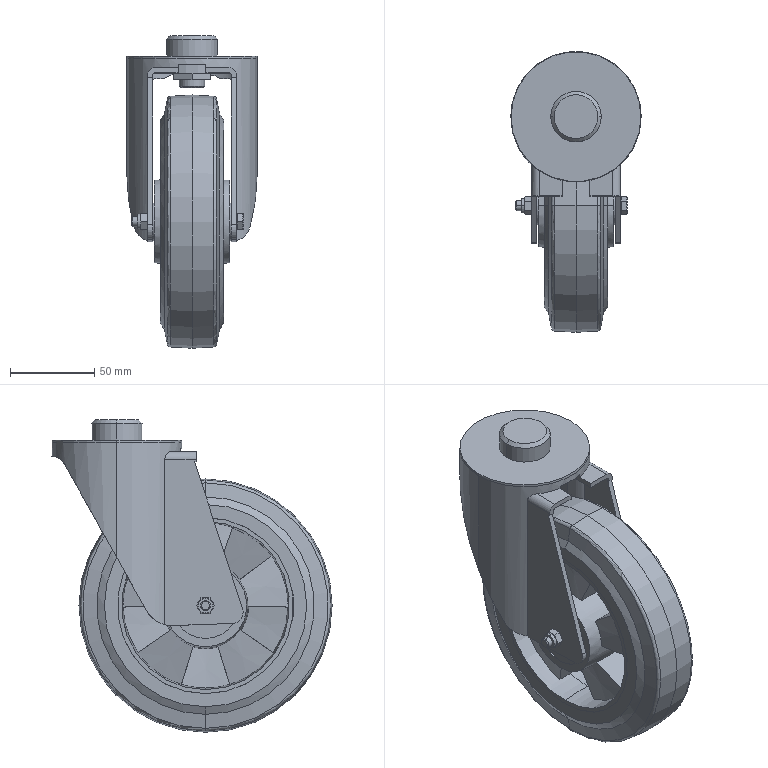Part | SolidWorks | features BaseBody 4, CombineBodies 2, ICE 2, Chamfer 1, MoveCopyBody 1, MoveFace 1, Scale 1 | 1 solid | 239 faces | box 77.25 x 166.125 x 185.063 mm | volume 534809 mm3 | plane 92 | cone 64 | cylinder 53 | torus 30 | commonest cylinder face diameters 6 x6 9 x6 8.723 x4 22.5 x4 34.5 x4 39 x4